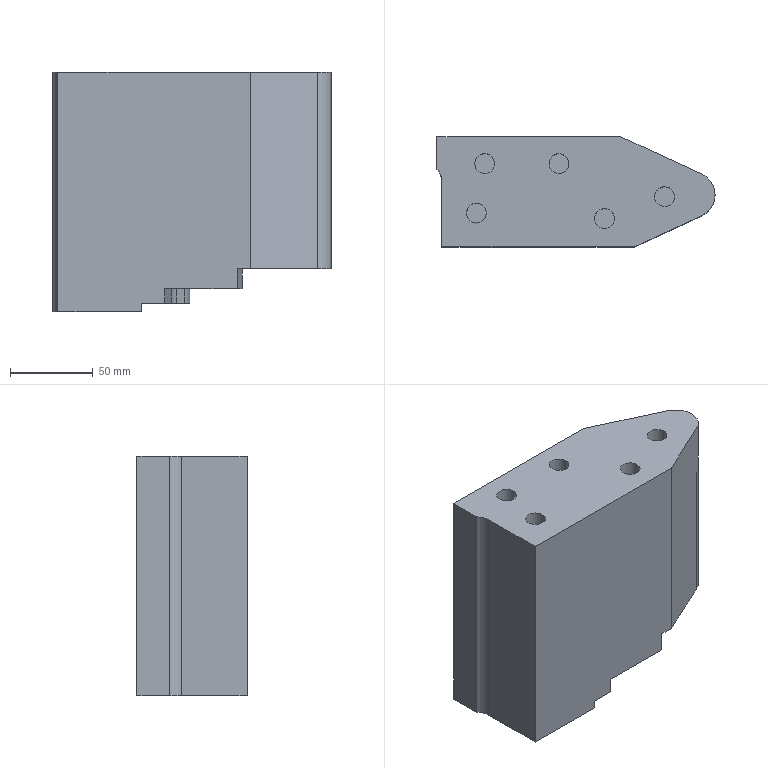Part | NX | features solid 2 | 1 solid | 34 faces | box 168.472 x 66.746 x 145 mm | volume 1281630 mm3 | plane 23 | cylinder 11 | commonest cylinder face diameters 12 x5 40 x4 20 x1 28 x1
STEP:
#1=CARTESIAN_POINT('',(645.,-7.,235.));
#2=VERTEX_POINT('',#1);
#3=CARTESIAN_POINT('',(645.,-13.,235.));
#4=DIRECTION('',(0.,0.,-1.));
#5=DIRECTION('',(0.,1.,0.));
#6=AXIS2_PLACEMENT_3D('',#3,#4,#5);
#7=CIRCLE('',#6,6.);
#8=EDGE_CURVE('',#2,#2,#7,.T.);
#9=ORIENTED_EDGE('',*,*,#8,.T.);
#10=EDGE_LOOP('',(#9));
#11=FACE_BOUND('',#10,.T.);
#12=CARTESIAN_POINT('',(650.,23.,235.));
#13=VERTEX_POINT('',#12);
#14=CARTESIAN_POINT('',(650.,17.,235.));
#15=DIRECTION('',(0.,0.,-1.));
#16=DIRECTION('',(0.,1.,0.));
#17=AXIS2_PLACEMENT_3D('',#14,#15,#16);
#18=CIRCLE('',#17,6.);
#19=EDGE_CURVE('',#13,#13,#18,.F.);
#20=ORIENTED_EDGE('',*,*,#19,.F.);
#21=EDGE_LOOP('',(#20));
#22=FACE_BOUND('',#21,.T.);
#23=CARTESIAN_POINT('',(695.,23.,235.));
#24=VERTEX_POINT('',#23);
#25=CARTESIAN_POINT('',(695.,17.,235.));
#26=DIRECTION('',(0.,0.,-1.));
#27=DIRECTION('',(0.,1.,0.));
#28=AXIS2_PLACEMENT_3D('',#25,#26,#27);
#29=CIRCLE('',#28,6.);
#30=EDGE_CURVE('',#24,#24,#29,.F.);
#31=ORIENTED_EDGE('',*,*,#30,.F.);
#32=EDGE_LOOP('',(#31));
#33=FACE_BOUND('',#32,.T.);
#34=CARTESIAN_POINT('',(722.608,-10.278,235.));
#35=VERTEX_POINT('',#34);
#36=CARTESIAN_POINT('',(722.608,-16.278,235.));
#37=DIRECTION('',(0.,0.,-1.));
#38=DIRECTION('',(0.,1.,0.));
#39=AXIS2_PLACEMENT_3D('',#36,#37,#38);
#40=CIRCLE('',#39,6.);
#41=EDGE_CURVE('',#35,#35,#40,.F.);
#42=ORIENTED_EDGE('',*,*,#41,.F.);
#43=EDGE_LOOP('',(#42));
#44=FACE_BOUND('',#43,.T.);
#45=CARTESIAN_POINT('',(759.,3.,235.));
#46=VERTEX_POINT('',#45);
#47=CARTESIAN_POINT('',(759.,-3.,235.));
#48=DIRECTION('',(0.,0.,-1.));
#49=DIRECTION('',(0.,1.,0.));
#50=AXIS2_PLACEMENT_3D('',#47,#48,#49);
#51=CIRCLE('',#50,6.);
#52=EDGE_CURVE('',#46,#46,#51,.F.);
#53=ORIENTED_EDGE('',*,*,#52,.F.);
#54=EDGE_LOOP('',(#53));
#55=FACE_BOUND('',#54,.T.);
#56=CARTESIAN_POINT('',(621.088,13.552,235.));
#57=VERTEX_POINT('',#56);
#58=CARTESIAN_POINT('',(621.088,33.298,235.));
#59=VERTEX_POINT('',#58);
#60=CARTESIAN_POINT('',(621.088,12.298,235.));
#61=DIRECTION('',(0.,1.,0.));
#62=VECTOR('',#61,1000.);
#63=LINE('',#60,#62);
#64=EDGE_CURVE('',#57,#59,#63,.T.);
#65=ORIENTED_EDGE('',*,*,#64,.F.);
#66=CARTESIAN_POINT('',(624.088,6.41,235.));
#67=VERTEX_POINT('',#66);
#68=CARTESIAN_POINT('',(614.088,6.41,235.));
#69=DIRECTION('',(0.,0.,-1.));
#70=DIRECTION('',(0.,1.,0.));
#71=AXIS2_PLACEMENT_3D('',#68,#69,#70);
#72=CIRCLE('',#71,10.);
#73=EDGE_CURVE('',#57,#67,#72,.T.);
#74=ORIENTED_EDGE('',*,*,#73,.T.);
#75=CARTESIAN_POINT('',(624.088,-33.448,235.));
#76=VERTEX_POINT('',#75);
#77=CARTESIAN_POINT('',(624.088,-164.676,235.));
#78=DIRECTION('',(0.,1.,0.));
#79=VECTOR('',#78,1000.);
#80=LINE('',#77,#79);
#81=EDGE_CURVE('',#67,#76,#80,.F.);
#82=ORIENTED_EDGE('',*,*,#81,.T.);
#83=CARTESIAN_POINT('',(740.626,-33.448,235.));
#84=VERTEX_POINT('',#83);
#85=CARTESIAN_POINT('',(-1135.,-33.448,235.));
#86=DIRECTION('',(-1.,0.,0.));
#87=VECTOR('',#86,1000.);
#88=LINE('',#85,#87);
#89=EDGE_CURVE('',#76,#84,#88,.F.);
#90=ORIENTED_EDGE('',*,*,#89,.T.);
#91=CARTESIAN_POINT('',(781.416,-14.665,235.));
#92=VERTEX_POINT('',#91);
#93=CARTESIAN_POINT('',(-856.712,-769.006,235.));
#94=DIRECTION('',(-0.9083,-0.4183,0.));
#95=VECTOR('',#94,1000.);
#96=LINE('',#93,#95);
#97=EDGE_CURVE('',#84,#92,#96,.F.);
#98=ORIENTED_EDGE('',*,*,#97,.T.);
#99=CARTESIAN_POINT('',(781.416,10.768,235.));
#100=VERTEX_POINT('',#99);
#101=CARTESIAN_POINT('',(775.56,-1.948,235.));
#102=DIRECTION('',(0.,0.,-1.));
#103=DIRECTION('',(0.,1.,0.));
#104=AXIS2_PLACEMENT_3D('',#101,#102,#103);
#105=CIRCLE('',#104,14.);
#106=EDGE_CURVE('',#92,#100,#105,.F.);
#107=ORIENTED_EDGE('',*,*,#106,.T.);
#108=CARTESIAN_POINT('',(732.491,33.298,235.));
#109=VERTEX_POINT('',#108);
#110=CARTESIAN_POINT('',(-733.063,708.17,235.));
#111=DIRECTION('',(0.9083,-0.4183,0.));
#112=VECTOR('',#111,1000.);
#113=LINE('',#110,#112);
#114=EDGE_CURVE('',#100,#109,#113,.F.);
#115=ORIENTED_EDGE('',*,*,#114,.T.);
#116=CARTESIAN_POINT('',(676.088,33.298,235.));
#117=DIRECTION('',(1.,0.,0.));
#118=VECTOR('',#117,1000.);
#119=LINE('',#116,#118);
#120=EDGE_CURVE('',#59,#109,#119,.T.);
#121=ORIENTED_EDGE('',*,*,#120,.F.);
#122=EDGE_LOOP('',(#65,#74,#82,#90,#98,#107,#115,#121));
#123=FACE_BOUND('',#122,.T.);
#124=CARTESIAN_POINT('',(-1135.,-164.676,235.));
#125=DIRECTION('',(0.,0.,-1.));
#126=DIRECTION('',(0.,1.,0.));
#127=AXIS2_PLACEMENT_3D('',#124,#125,#126);
#128=PLANE('',#127);
#129=ADVANCED_FACE('',(#11,#22,#33,#44,#55,#123),#128,.F.);
#130=ORIENTED_EDGE('',*,*,#89,.F.);
#131=CARTESIAN_POINT('',(624.088,-33.448,90.));
#132=VERTEX_POINT('',#131);
#133=CARTESIAN_POINT('',(624.088,-33.448,-185.));
#134=DIRECTION('',(0.,0.,1.));
#135=VECTOR('',#134,1000.);
#136=LINE('',#133,#135);
#137=EDGE_CURVE('',#132,#76,#136,.T.);
#138=ORIENTED_EDGE('',*,*,#137,.F.);
#139=CARTESIAN_POINT('',(674.638,-33.448,90.));
#140=VERTEX_POINT('',#139);
#141=CARTESIAN_POINT('',(621.088,-33.448,90.));
#142=DIRECTION('',(1.,0.,0.));
#143=VECTOR('',#142,1000.);
#144=LINE('',#141,#143);
#145=EDGE_CURVE('',#132,#140,#144,.T.);
#146=ORIENTED_EDGE('',*,*,#145,.T.);
#147=CARTESIAN_POINT('',(674.638,-33.448,95.));
#148=VERTEX_POINT('',#147);
#149=CARTESIAN_POINT('',(674.638,-33.448,95.));
#150=DIRECTION('',(0.,0.,-1.));
#151=VECTOR('',#150,1000.);
#152=LINE('',#149,#151);
#153=EDGE_CURVE('',#148,#140,#152,.T.);
#154=ORIENTED_EDGE('',*,*,#153,.F.);
#155=CARTESIAN_POINT('',(688.816,-33.448,95.));
#156=VERTEX_POINT('',#155);
#157=CARTESIAN_POINT('',(684.588,-33.448,95.));
#158=DIRECTION('',(1.,0.,0.));
#159=VECTOR('',#158,1000.);
#160=LINE('',#157,#159);
#161=EDGE_CURVE('',#148,#156,#160,.T.);
#162=ORIENTED_EDGE('',*,*,#161,.T.);
#163=CARTESIAN_POINT('',(688.816,-33.448,104.));
#164=VERTEX_POINT('',#163);
#165=CARTESIAN_POINT('',(688.816,-33.448,81.));
#166=DIRECTION('',(0.,0.,1.));
#167=VECTOR('',#166,1000.);
#168=LINE('',#165,#167);
#169=EDGE_CURVE('',#156,#164,#168,.T.);
#170=ORIENTED_EDGE('',*,*,#169,.T.);
#171=CARTESIAN_POINT('',(732.667,-33.448,104.));
#172=VERTEX_POINT('',#171);
#173=CARTESIAN_POINT('',(737.56,-33.448,104.));
#174=DIRECTION('',(-1.,0.,0.));
#175=VECTOR('',#174,1000.);
#176=LINE('',#173,#175);
#177=EDGE_CURVE('',#164,#172,#176,.F.);
#178=ORIENTED_EDGE('',*,*,#177,.T.);
#179=CARTESIAN_POINT('',(732.667,-33.448,116.));
#180=VERTEX_POINT('',#179);
#181=CARTESIAN_POINT('',(732.667,-33.448,81.));
#182=DIRECTION('',(0.,0.,1.));
#183=VECTOR('',#182,1000.);
#184=LINE('',#181,#183);
#185=EDGE_CURVE('',#172,#180,#184,.T.);
#186=ORIENTED_EDGE('',*,*,#185,.T.);
#187=CARTESIAN_POINT('',(740.626,-33.448,116.));
#188=VERTEX_POINT('',#187);
#189=CARTESIAN_POINT('',(737.56,-33.448,116.));
#190=DIRECTION('',(-1.,0.,0.));
#191=VECTOR('',#190,1000.);
#192=LINE('',#189,#191);
#193=EDGE_CURVE('',#180,#188,#192,.F.);
#194=ORIENTED_EDGE('',*,*,#193,.T.);
#195=CARTESIAN_POINT('',(740.626,-33.448,81.));
#196=DIRECTION('',(0.,0.,1.));
#197=VECTOR('',#196,1000.);
#198=LINE('',#195,#197);
#199=EDGE_CURVE('',#188,#84,#198,.T.);
#200=ORIENTED_EDGE('',*,*,#199,.T.);
#201=EDGE_LOOP('',(#130,#138,#146,#154,#162,#170,#178,#186,#194,#200));
#202=FACE_BOUND('',#201,.T.);
#203=CARTESIAN_POINT('',(737.56,-33.448,81.));
#204=DIRECTION('',(0.,-1.,0.));
#205=DIRECTION('',(0.,0.,1.));
#206=AXIS2_PLACEMENT_3D('',#203,#204,#205);
#207=PLANE('',#206);
#208=ADVANCED_FACE('',(#202),#207,.T.);
#209=CARTESIAN_POINT('',(621.088,13.552,90.));
#210=VERTEX_POINT('',#209);
#211=CARTESIAN_POINT('',(621.088,33.298,90.));
#212=VERTEX_POINT('',#211);
#213=CARTESIAN_POINT('',(621.088,-33.448,90.));
#214=DIRECTION('',(0.,1.,0.));
#215=VECTOR('',#214,1000.);
#216=LINE('',#213,#215);
#217=EDGE_CURVE('',#210,#212,#216,.T.);
#218=ORIENTED_EDGE('',*,*,#217,.F.);
#219=CARTESIAN_POINT('',(621.088,13.552,-185.));
#220=DIRECTION('',(0.,0.,1.));
#221=VECTOR('',#220,1000.);
#222=LINE('',#219,#221);
#223=EDGE_CURVE('',#210,#57,#222,.T.);
#224=ORIENTED_EDGE('',*,*,#223,.T.);
#225=ORIENTED_EDGE('',*,*,#64,.T.);
#226=CARTESIAN_POINT('',(621.088,33.298,95.));
#227=DIRECTION('',(0.,0.,1.));
#228=VECTOR('',#227,1000.);
#229=LINE('',#226,#228);
#230=EDGE_CURVE('',#212,#59,#229,.T.);
#231=ORIENTED_EDGE('',*,*,#230,.F.);
#232=EDGE_LOOP('',(#218,#224,#225,#231));
#233=FACE_BOUND('',#232,.T.);
#234=CARTESIAN_POINT('',(621.088,12.298,95.));
#235=DIRECTION('',(1.,0.,0.));
#236=DIRECTION('',(0.,1.,0.));
#237=AXIS2_PLACEMENT_3D('',#234,#235,#236);
#238=PLANE('',#237);
#239=ADVANCED_FACE('',(#233),#238,.F.);
#240=CARTESIAN_POINT('',(624.088,6.41,90.));
#241=VERTEX_POINT('',#240);
#242=CARTESIAN_POINT('',(614.088,6.41,90.));
#243=DIRECTION('',(0.,0.,1.));
#244=DIRECTION('',(1.,0.,0.));
#245=AXIS2_PLACEMENT_3D('',#242,#243,#244);
#246=CIRCLE('',#245,10.);
#247=EDGE_CURVE('',#210,#241,#246,.F.);
#248=ORIENTED_EDGE('',*,*,#247,.F.);
#249=ORIENTED_EDGE('',*,*,#217,.T.);
#250=CARTESIAN_POINT('',(650.299,33.298,90.));
#251=VERTEX_POINT('',#250);
#252=CARTESIAN_POINT('',(621.088,33.298,90.));
#253=DIRECTION('',(1.,0.,0.));
#254=VECTOR('',#253,1000.);
#255=LINE('',#252,#254);
#256=EDGE_CURVE('',#212,#251,#255,.T.);
#257=ORIENTED_EDGE('',*,*,#256,.T.);
#258=CARTESIAN_POINT('',(664.3,13.301,90.));
#259=VERTEX_POINT('',#258);
#260=CARTESIAN_POINT('',(649.897,33.871,90.));
#261=DIRECTION('',(0.5736,-0.8192,0.));
#262=VECTOR('',#261,1000.);
#263=LINE('',#260,#262);
#264=EDGE_CURVE('',#251,#259,#263,.T.);
#265=ORIENTED_EDGE('',*,*,#264,.T.);
#266=CARTESIAN_POINT('',(667.597,5.397,90.));
#267=VERTEX_POINT('',#266);
#268=CARTESIAN_POINT('',(647.917,1.829,90.));
#269=DIRECTION('',(0.,0.,1.));
#270=DIRECTION('',(1.,0.,0.));
#271=AXIS2_PLACEMENT_3D('',#268,#269,#270);
#272=CIRCLE('',#271,20.);
#273=EDGE_CURVE('',#259,#267,#272,.F.);
#274=ORIENTED_EDGE('',*,*,#273,.T.);
#275=CARTESIAN_POINT('',(666.854,9.494,90.));
#276=DIRECTION('',(0.1784,-0.984,0.));
#277=VECTOR('',#276,1000.);
#278=LINE('',#275,#277);
#279=EDGE_CURVE('',#267,#140,#278,.T.);
#280=ORIENTED_EDGE('',*,*,#279,.T.);
#281=ORIENTED_EDGE('',*,*,#145,.F.);
#282=CARTESIAN_POINT('',(624.088,-33.448,90.));
#283=DIRECTION('',(0.,-1.,0.));
#284=VECTOR('',#283,1000.);
#285=LINE('',#282,#284);
#286=EDGE_CURVE('',#241,#132,#285,.T.);
#287=ORIENTED_EDGE('',*,*,#286,.F.);
#288=EDGE_LOOP('',(#248,#249,#257,#265,#274,#280,#281,#287));
#289=FACE_BOUND('',#288,.T.);
#290=CARTESIAN_POINT('',(621.088,-33.448,90.));
#291=DIRECTION('',(0.,0.,1.));
#292=DIRECTION('',(1.,0.,0.));
#293=AXIS2_PLACEMENT_3D('',#290,#291,#292);
#294=PLANE('',#293);
#295=ADVANCED_FACE('',(#289),#294,.F.);
#296=CARTESIAN_POINT('',(704.088,33.298,95.));
#297=VERTEX_POINT('',#296);
#298=CARTESIAN_POINT('',(704.088,17.136,95.));
#299=VERTEX_POINT('',#298);
#300=CARTESIAN_POINT('',(704.088,-2.702,95.));
#301=DIRECTION('',(0.,-1.,0.));
#302=VECTOR('',#301,1000.);
#303=LINE('',#300,#302);
#304=EDGE_CURVE('',#297,#299,#303,.T.);
#305=ORIENTED_EDGE('',*,*,#304,.T.);
#306=CARTESIAN_POINT('',(700.722,6.031,95.));
#307=VERTEX_POINT('',#306);
#308=CARTESIAN_POINT('',(684.088,17.136,95.));
#309=DIRECTION('',(0.,0.,1.));
#310=DIRECTION('',(1.,0.,0.));
#311=AXIS2_PLACEMENT_3D('',#308,#309,#310);
#312=CIRCLE('',#311,20.);
#313=EDGE_CURVE('',#299,#307,#312,.F.);
#314=ORIENTED_EDGE('',*,*,#313,.T.);
#315=CARTESIAN_POINT('',(695.744,-1.427,95.));
#316=VERTEX_POINT('',#315);
#317=CARTESIAN_POINT('',(691.716,-7.46,95.));
#318=DIRECTION('',(0.5552,0.8317,0.));
#319=VECTOR('',#318,1000.);
#320=LINE('',#317,#319);
#321=EDGE_CURVE('',#316,#307,#320,.T.);
#322=ORIENTED_EDGE('',*,*,#321,.F.);
#323=CARTESIAN_POINT('',(692.624,-9.402,95.));
#324=VERTEX_POINT('',#323);
#325=CARTESIAN_POINT('',(712.378,-12.531,95.));
#326=DIRECTION('',(0.,0.,1.));
#327=DIRECTION('',(1.,0.,0.));
#328=AXIS2_PLACEMENT_3D('',#325,#326,#327);
#329=CIRCLE('',#328,20.);
#330=EDGE_CURVE('',#316,#324,#329,.T.);
#331=ORIENTED_EDGE('',*,*,#330,.T.);
#332=CARTESIAN_POINT('',(693.463,-4.108,95.));
#333=DIRECTION('',(0.1564,0.9877,0.));
#334=VECTOR('',#333,1000.);
#335=LINE('',#332,#334);
#336=EDGE_CURVE('',#156,#324,#335,.T.);
#337=ORIENTED_EDGE('',*,*,#336,.F.);
#338=ORIENTED_EDGE('',*,*,#161,.F.);
#339=CARTESIAN_POINT('',(667.597,5.397,95.));
#340=VERTEX_POINT('',#339);
#341=CARTESIAN_POINT('',(666.854,9.494,95.));
#342=DIRECTION('',(0.1784,-0.984,0.));
#343=VECTOR('',#342,1000.);
#344=LINE('',#341,#343);
#345=EDGE_CURVE('',#340,#148,#344,.T.);
#346=ORIENTED_EDGE('',*,*,#345,.F.);
#347=CARTESIAN_POINT('',(664.3,13.301,95.));
#348=VERTEX_POINT('',#347);
#349=CARTESIAN_POINT('',(647.917,1.829,95.));
#350=DIRECTION('',(0.,0.,1.));
#351=DIRECTION('',(1.,0.,0.));
#352=AXIS2_PLACEMENT_3D('',#349,#350,#351);
#353=CIRCLE('',#352,20.);
#354=EDGE_CURVE('',#340,#348,#353,.T.);
#355=ORIENTED_EDGE('',*,*,#354,.T.);
#356=CARTESIAN_POINT('',(650.299,33.298,95.));
#357=VERTEX_POINT('',#356);
#358=CARTESIAN_POINT('',(649.897,33.871,95.));
#359=DIRECTION('',(0.5736,-0.8192,0.));
#360=VECTOR('',#359,1000.);
#361=LINE('',#358,#360);
#362=EDGE_CURVE('',#357,#348,#361,.T.);
#363=ORIENTED_EDGE('',*,*,#362,.F.);
#364=CARTESIAN_POINT('',(676.088,33.298,95.));
#365=DIRECTION('',(-1.,0.,0.));
#366=VECTOR('',#365,1000.);
#367=LINE('',#364,#366);
#368=EDGE_CURVE('',#357,#297,#367,.F.);
#369=ORIENTED_EDGE('',*,*,#368,.T.);
#370=EDGE_LOOP('',(#305,#314,#322,#331,#337,#338,#346,#355,#363,#369));
#371=FACE_BOUND('',#370,.T.);
#372=CARTESIAN_POINT('',(684.588,-2.702,95.));
#373=DIRECTION('',(0.,0.,1.));
#374=DIRECTION('',(0.,1.,0.));
#375=AXIS2_PLACEMENT_3D('',#372,#373,#374);
#376=PLANE('',#375);
#377=ADVANCED_FACE('',(#371),#376,.F.);
#378=CARTESIAN_POINT('',(704.088,33.298,104.));
#379=VERTEX_POINT('',#378);
#380=CARTESIAN_POINT('',(704.088,33.298,95.));
#381=DIRECTION('',(0.,0.,-1.));
#382=VECTOR('',#381,1000.);
#383=LINE('',#380,#382);
#384=EDGE_CURVE('',#297,#379,#383,.F.);
#385=ORIENTED_EDGE('',*,*,#384,.F.);
#386=ORIENTED_EDGE('',*,*,#368,.F.);
#387=CARTESIAN_POINT('',(650.299,33.298,95.));
#388=DIRECTION('',(0.,0.,-1.));
#389=VECTOR('',#388,1000.);
#390=LINE('',#387,#389);
#391=EDGE_CURVE('',#357,#251,#390,.T.);
#392=ORIENTED_EDGE('',*,*,#391,.T.);
#393=ORIENTED_EDGE('',*,*,#256,.F.);
#394=ORIENTED_EDGE('',*,*,#230,.T.);
#395=ORIENTED_EDGE('',*,*,#120,.T.);
#396=CARTESIAN_POINT('',(732.491,33.298,116.));
#397=VERTEX_POINT('',#396);
#398=CARTESIAN_POINT('',(732.491,33.298,95.));
#399=DIRECTION('',(0.,0.,1.));
#400=VECTOR('',#399,1000.);
#401=LINE('',#398,#400);
#402=EDGE_CURVE('',#109,#397,#401,.F.);
#403=ORIENTED_EDGE('',*,*,#402,.T.);
#404=CARTESIAN_POINT('',(724.328,33.298,116.));
#405=VERTEX_POINT('',#404);
#406=CARTESIAN_POINT('',(676.088,33.298,116.));
#407=DIRECTION('',(-1.,0.,0.));
#408=VECTOR('',#407,1000.);
#409=LINE('',#406,#408);
#410=EDGE_CURVE('',#405,#397,#409,.F.);
#411=ORIENTED_EDGE('',*,*,#410,.F.);
#412=CARTESIAN_POINT('',(724.328,33.298,104.));
#413=VERTEX_POINT('',#412);
#414=CARTESIAN_POINT('',(724.328,33.298,95.));
#415=DIRECTION('',(0.,0.,1.));
#416=VECTOR('',#415,1000.);
#417=LINE('',#414,#416);
#418=EDGE_CURVE('',#413,#405,#417,.T.);
#419=ORIENTED_EDGE('',*,*,#418,.F.);
#420=CARTESIAN_POINT('',(718.314,33.298,104.));
#421=DIRECTION('',(1.,0.,0.));
#422=VECTOR('',#421,1000.);
#423=LINE('',#420,#422);
#424=EDGE_CURVE('',#379,#413,#423,.T.);
#425=ORIENTED_EDGE('',*,*,#424,.F.);
#426=EDGE_LOOP('',(#385,#386,#392,#393,#394,#395,#403,#411,#419,#425));
#427=FACE_BOUND('',#426,.T.);
#428=CARTESIAN_POINT('',(676.088,33.298,95.));
#429=DIRECTION('',(0.,-1.,0.));
#430=DIRECTION('',(1.,0.,0.));
#431=AXIS2_PLACEMENT_3D('',#428,#429,#430);
#432=PLANE('',#431);
#433=ADVANCED_FACE('',(#427),#432,.F.);
#434=CARTESIAN_POINT('',(781.416,-14.665,116.));
#435=VERTEX_POINT('',#434);
#436=CARTESIAN_POINT('',(781.416,-14.665,-270.));
#437=DIRECTION('',(0.,0.,1.));
#438=VECTOR('',#437,1000.);
#439=LINE('',#436,#438);
#440=EDGE_CURVE('',#435,#92,#439,.T.);
#441=ORIENTED_EDGE('',*,*,#440,.F.);
#442=CARTESIAN_POINT('',(781.416,10.768,116.));
#443=VERTEX_POINT('',#442);
#444=CARTESIAN_POINT('',(775.56,-1.948,116.));
#445=DIRECTION('',(0.,0.,1.));
#446=DIRECTION('',(1.,0.,0.));
#447=AXIS2_PLACEMENT_3D('',#444,#445,#446);
#448=CIRCLE('',#447,14.);
#449=EDGE_CURVE('',#435,#443,#448,.T.);
#450=ORIENTED_EDGE('',*,*,#449,.T.);
#451=CARTESIAN_POINT('',(781.416,10.768,-270.));
#452=DIRECTION('',(0.,0.,1.));
#453=VECTOR('',#452,1000.);
#454=LINE('',#451,#453);
#455=EDGE_CURVE('',#443,#100,#454,.T.);
#456=ORIENTED_EDGE('',*,*,#455,.T.);
#457=ORIENTED_EDGE('',*,*,#106,.F.);
#458=EDGE_LOOP('',(#441,#450,#456,#457));
#459=FACE_BOUND('',#458,.T.);
#460=CARTESIAN_POINT('',(775.56,-1.948,-270.));
#461=DIRECTION('',(0.,0.,1.));
#462=DIRECTION('',(1.,0.,0.));
#463=AXIS2_PLACEMENT_3D('',#460,#461,#462);
#464=CYLINDRICAL_SURFACE('',#463,14.);
#465=ADVANCED_FACE('',(#459),#464,.T.);
#466=CARTESIAN_POINT('',(758.397,21.368,116.));
#467=DIRECTION('',(-0.9083,0.4183,0.));
#468=VECTOR('',#467,1000.);
#469=LINE('',#466,#468);
#470=EDGE_CURVE('',#397,#443,#469,.F.);
#471=ORIENTED_EDGE('',*,*,#470,.F.);
#472=ORIENTED_EDGE('',*,*,#402,.F.);
#473=ORIENTED_EDGE('',*,*,#114,.F.);
#474=ORIENTED_EDGE('',*,*,#455,.F.);
#475=EDGE_LOOP('',(#471,#472,#473,#474));
#476=FACE_BOUND('',#475,.T.);
#477=CARTESIAN_POINT('',(781.416,10.768,-270.));
#478=DIRECTION('',(0.4183,0.9083,0.));
#479=DIRECTION('',(-0.9083,0.4183,0.));
#480=AXIS2_PLACEMENT_3D('',#477,#478,#479);
#481=PLANE('',#480);
#482=ADVANCED_FACE('',(#476),#481,.T.);
#483=ORIENTED_EDGE('',*,*,#199,.F.);
#484=CARTESIAN_POINT('',(781.416,-14.665,116.));
#485=DIRECTION('',(0.9083,0.4183,0.));
#486=VECTOR('',#485,1000.);
#487=LINE('',#484,#486);
#488=EDGE_CURVE('',#435,#188,#487,.F.);
#489=ORIENTED_EDGE('',*,*,#488,.F.);
#490=ORIENTED_EDGE('',*,*,#440,.T.);
#491=ORIENTED_EDGE('',*,*,#97,.F.);
#492=EDGE_LOOP('',(#483,#489,#490,#491));
#493=FACE_BOUND('',#492,.T.);
#494=CARTESIAN_POINT('',(736.614,-35.296,-270.));
#495=DIRECTION('',(0.4183,-0.9083,0.));
#496=DIRECTION('',(0.9083,0.4183,0.));
#497=AXIS2_PLACEMENT_3D('',#494,#495,#496);
#498=PLANE('',#497);
#499=ADVANCED_FACE('',(#493),#498,.T.);
#500=CARTESIAN_POINT('',(735.601,-16.808,104.));
#501=VERTEX_POINT('',#500);
#502=CARTESIAN_POINT('',(735.248,-8.251,104.));
#503=VERTEX_POINT('',#502);
#504=CARTESIAN_POINT('',(715.905,-13.335,104.));
#505=DIRECTION('',(0.,0.,1.));
#506=DIRECTION('',(1.,0.,0.));
#507=AXIS2_PLACEMENT_3D('',#504,#505,#506);
#508=CIRCLE('',#507,20.);
#509=EDGE_CURVE('',#501,#503,#508,.T.);
#510=ORIENTED_EDGE('',*,*,#509,.T.);
#511=CARTESIAN_POINT('',(735.248,-8.251,116.));
#512=VERTEX_POINT('',#511);
#513=CARTESIAN_POINT('',(735.248,-8.251,-384.));
#514=DIRECTION('',(0.,0.,1.));
#515=VECTOR('',#514,1000.);
#516=LINE('',#513,#515);
#517=EDGE_CURVE('',#503,#512,#516,.T.);
#518=ORIENTED_EDGE('',*,*,#517,.T.);
#519=CARTESIAN_POINT('',(735.601,-16.808,116.));
#520=VERTEX_POINT('',#519);
#521=CARTESIAN_POINT('',(715.905,-13.335,116.));
#522=DIRECTION('',(0.,0.,1.));
#523=DIRECTION('',(1.,0.,0.));
#524=AXIS2_PLACEMENT_3D('',#521,#522,#523);
#525=CIRCLE('',#524,20.);
#526=EDGE_CURVE('',#520,#512,#525,.T.);
#527=ORIENTED_EDGE('',*,*,#526,.F.);
#528=CARTESIAN_POINT('',(735.601,-16.808,-384.));
#529=DIRECTION('',(0.,0.,1.));
#530=VECTOR('',#529,1000.);
#531=LINE('',#528,#530);
#532=EDGE_CURVE('',#501,#520,#531,.T.);
#533=ORIENTED_EDGE('',*,*,#532,.F.);
#534=EDGE_LOOP('',(#510,#518,#527,#533));
#535=FACE_BOUND('',#534,.T.);
#536=CARTESIAN_POINT('',(715.905,-13.335,-384.));
#537=DIRECTION('',(0.,0.,1.));
#538=DIRECTION('',(1.,0.,0.));
#539=AXIS2_PLACEMENT_3D('',#536,#537,#538);
#540=CYLINDRICAL_SURFACE('',#539,20.);
#541=ADVANCED_FACE('',(#535),#540,.T.);
#542=CARTESIAN_POINT('',(736.303,-12.266,104.));
#543=DIRECTION('',(0.2542,-0.9672,0.));
#544=VECTOR('',#543,1000.);
#545=LINE('',#542,#544);
#546=EDGE_CURVE('',#503,#413,#545,.F.);
#547=ORIENTED_EDGE('',*,*,#546,.T.);
#548=ORIENTED_EDGE('',*,*,#418,.T.);
#549=CARTESIAN_POINT('',(736.303,-12.266,116.));
#550=DIRECTION('',(0.2542,-0.9672,0.));
#551=VECTOR('',#550,1000.);
#552=LINE('',#549,#551);
#553=EDGE_CURVE('',#512,#405,#552,.F.);
#554=ORIENTED_EDGE('',*,*,#553,.F.);
#555=ORIENTED_EDGE('',*,*,#517,.F.);
#556=EDGE_LOOP('',(#547,#548,#554,#555));
#557=FACE_BOUND('',#556,.T.);
#558=CARTESIAN_POINT('',(736.303,-12.266,-384.));
#559=DIRECTION('',(0.9672,0.2542,0.));
#560=DIRECTION('',(-0.2542,0.9672,0.));
#561=AXIS2_PLACEMENT_3D('',#558,#559,#560);
#562=PLANE('',#561);
#563=ADVANCED_FACE('',(#557),#562,.T.);
#564=CARTESIAN_POINT('',(739.347,4.437,104.));
#565=DIRECTION('',(-0.1736,-0.9848,0.));
#566=VECTOR('',#565,1000.);
#567=LINE('',#564,#566);
#568=EDGE_CURVE('',#172,#501,#567,.F.);
#569=ORIENTED_EDGE('',*,*,#568,.T.);
#570=ORIENTED_EDGE('',*,*,#532,.T.);
#571=CARTESIAN_POINT('',(739.347,4.437,116.));
#572=DIRECTION('',(-0.1736,-0.9848,0.));
#573=VECTOR('',#572,1000.);
#574=LINE('',#571,#573);
#575=EDGE_CURVE('',#180,#520,#574,.F.);
#576=ORIENTED_EDGE('',*,*,#575,.F.);
#577=ORIENTED_EDGE('',*,*,#185,.F.);
#578=EDGE_LOOP('',(#569,#570,#576,#577));
#579=FACE_BOUND('',#578,.T.);
#580=CARTESIAN_POINT('',(739.347,4.437,-384.));
#581=DIRECTION('',(0.9848,-0.1736,0.));
#582=DIRECTION('',(0.1736,0.9848,0.));
#583=AXIS2_PLACEMENT_3D('',#580,#581,#582);
#584=PLANE('',#583);
#585=ADVANCED_FACE('',(#579),#584,.T.);
#586=ORIENTED_EDGE('',*,*,#575,.T.);
#587=ORIENTED_EDGE('',*,*,#526,.T.);
#588=ORIENTED_EDGE('',*,*,#553,.T.);
#589=ORIENTED_EDGE('',*,*,#410,.T.);
#590=ORIENTED_EDGE('',*,*,#470,.T.);
#591=ORIENTED_EDGE('',*,*,#449,.F.);
#592=ORIENTED_EDGE('',*,*,#488,.T.);
#593=ORIENTED_EDGE('',*,*,#193,.F.);
#594=EDGE_LOOP('',(#586,#587,#588,#589,#590,#591,#592,#593));
#595=FACE_BOUND('',#594,.T.);
#596=CARTESIAN_POINT('',(775.56,-1.948,116.));
#597=DIRECTION('',(0.,0.,1.));
#598=DIRECTION('',(-1.,0.,0.));
#599=AXIS2_PLACEMENT_3D('',#596,#597,#598);
#600=PLANE('',#599);
#601=ADVANCED_FACE('',(#595),#600,.F.);
#602=ORIENTED_EDGE('',*,*,#279,.F.);
#603=CARTESIAN_POINT('',(667.597,5.397,95.));
#604=DIRECTION('',(0.,0.,-1.));
#605=VECTOR('',#604,1000.);
#606=LINE('',#603,#605);
#607=EDGE_CURVE('',#267,#340,#606,.F.);
#608=ORIENTED_EDGE('',*,*,#607,.T.);
#609=ORIENTED_EDGE('',*,*,#345,.T.);
#610=ORIENTED_EDGE('',*,*,#153,.T.);
#611=EDGE_LOOP('',(#602,#608,#609,#610));
#612=FACE_BOUND('',#611,.T.);
#613=CARTESIAN_POINT('',(666.854,9.494,95.));
#614=DIRECTION('',(0.984,0.1784,0.));
#615=DIRECTION('',(-0.1784,0.984,0.));
#616=AXIS2_PLACEMENT_3D('',#613,#614,#615);
#617=PLANE('',#616);
#618=ADVANCED_FACE('',(#612),#617,.T.);
#619=ORIENTED_EDGE('',*,*,#362,.T.);
#620=CARTESIAN_POINT('',(664.3,13.301,95.));
#621=DIRECTION('',(0.,0.,-1.));
#622=VECTOR('',#621,1000.);
#623=LINE('',#620,#622);
#624=EDGE_CURVE('',#348,#259,#623,.T.);
#625=ORIENTED_EDGE('',*,*,#624,.T.);
#626=ORIENTED_EDGE('',*,*,#264,.F.);
#627=ORIENTED_EDGE('',*,*,#391,.F.);
#628=EDGE_LOOP('',(#619,#625,#626,#627));
#629=FACE_BOUND('',#628,.T.);
#630=CARTESIAN_POINT('',(649.897,33.871,95.));
#631=DIRECTION('',(0.8192,0.5736,0.));
#632=DIRECTION('',(-0.5736,0.8192,0.));
#633=AXIS2_PLACEMENT_3D('',#630,#631,#632);
#634=PLANE('',#633);
#635=ADVANCED_FACE('',(#629),#634,.T.);
#636=ORIENTED_EDGE('',*,*,#354,.F.);
#637=ORIENTED_EDGE('',*,*,#607,.F.);
#638=ORIENTED_EDGE('',*,*,#273,.F.);
#639=ORIENTED_EDGE('',*,*,#624,.F.);
#640=EDGE_LOOP('',(#636,#637,#638,#639));
#641=FACE_BOUND('',#640,.T.);
#642=CARTESIAN_POINT('',(647.917,1.829,95.));
#643=DIRECTION('',(0.,0.,-1.));
#644=DIRECTION('',(-1.,0.,0.));
#645=AXIS2_PLACEMENT_3D('',#642,#643,#644);
#646=CYLINDRICAL_SURFACE('',#645,20.);
#647=ADVANCED_FACE('',(#641),#646,.T.);
#648=ORIENTED_EDGE('',*,*,#336,.T.);
#649=CARTESIAN_POINT('',(692.624,-9.402,104.));
#650=VERTEX_POINT('',#649);
#651=CARTESIAN_POINT('',(692.624,-9.402,104.));
#652=DIRECTION('',(0.,0.,1.));
#653=VECTOR('',#652,1000.);
#654=LINE('',#651,#653);
#655=EDGE_CURVE('',#324,#650,#654,.T.);
#656=ORIENTED_EDGE('',*,*,#655,.T.);
#657=CARTESIAN_POINT('',(688.84,-33.292,104.));
#658=DIRECTION('',(-0.1564,-0.9877,0.));
#659=VECTOR('',#658,1000.);
#660=LINE('',#657,#659);
#661=EDGE_CURVE('',#164,#650,#660,.F.);
#662=ORIENTED_EDGE('',*,*,#661,.F.);
#663=ORIENTED_EDGE('',*,*,#169,.F.);
#664=EDGE_LOOP('',(#648,#656,#662,#663));
#665=FACE_BOUND('',#664,.T.);
#666=CARTESIAN_POINT('',(688.84,-33.292,95.));
#667=DIRECTION('',(0.9877,-0.1564,0.));
#668=DIRECTION('',(0.1564,0.9877,0.));
#669=AXIS2_PLACEMENT_3D('',#666,#667,#668);
#670=PLANE('',#669);
#671=ADVANCED_FACE('',(#665),#670,.T.);
#672=ORIENTED_EDGE('',*,*,#321,.T.);
#673=CARTESIAN_POINT('',(700.722,6.031,104.));
#674=VERTEX_POINT('',#673);
#675=CARTESIAN_POINT('',(700.722,6.031,104.));
#676=DIRECTION('',(0.,0.,1.));
#677=VECTOR('',#676,1000.);
#678=LINE('',#675,#677);
#679=EDGE_CURVE('',#307,#674,#678,.T.);
#680=ORIENTED_EDGE('',*,*,#679,.T.);
#681=CARTESIAN_POINT('',(695.744,-1.427,104.));
#682=VERTEX_POINT('',#681);
#683=CARTESIAN_POINT('',(693.432,-4.89,104.));
#684=DIRECTION('',(-0.5552,-0.8317,0.));
#685=VECTOR('',#684,1000.);
#686=LINE('',#683,#685);
#687=EDGE_CURVE('',#682,#674,#686,.F.);
#688=ORIENTED_EDGE('',*,*,#687,.F.);
#689=CARTESIAN_POINT('',(695.744,-1.427,95.));
#690=DIRECTION('',(0.,0.,1.));
#691=VECTOR('',#690,1000.);
#692=LINE('',#689,#691);
#693=EDGE_CURVE('',#682,#316,#692,.F.);
#694=ORIENTED_EDGE('',*,*,#693,.T.);
#695=EDGE_LOOP('',(#672,#680,#688,#694));
#696=FACE_BOUND('',#695,.T.);
#697=CARTESIAN_POINT('',(693.432,-4.89,95.));
#698=DIRECTION('',(0.8317,-0.5552,0.));
#699=DIRECTION('',(0.5552,0.8317,0.));
#700=AXIS2_PLACEMENT_3D('',#697,#698,#699);
#701=PLANE('',#700);
#702=ADVANCED_FACE('',(#696),#701,.T.);
#703=ORIENTED_EDGE('',*,*,#661,.T.);
#704=CARTESIAN_POINT('',(712.378,-12.531,104.));
#705=DIRECTION('',(0.,0.,1.));
#706=DIRECTION('',(1.,0.,0.));
#707=AXIS2_PLACEMENT_3D('',#704,#705,#706);
#708=CIRCLE('',#707,20.);
#709=EDGE_CURVE('',#650,#682,#708,.F.);
#710=ORIENTED_EDGE('',*,*,#709,.T.);
#711=ORIENTED_EDGE('',*,*,#687,.T.);
#712=CARTESIAN_POINT('',(704.088,17.136,104.));
#713=VERTEX_POINT('',#712);
#714=CARTESIAN_POINT('',(684.088,17.136,104.));
#715=DIRECTION('',(0.,0.,1.));
#716=DIRECTION('',(1.,0.,0.));
#717=AXIS2_PLACEMENT_3D('',#714,#715,#716);
#718=CIRCLE('',#717,20.);
#719=EDGE_CURVE('',#674,#713,#718,.T.);
#720=ORIENTED_EDGE('',*,*,#719,.T.);
#721=CARTESIAN_POINT('',(704.088,33.298,104.));
#722=DIRECTION('',(0.,1.,0.));
#723=VECTOR('',#722,1000.);
#724=LINE('',#721,#723);
#725=EDGE_CURVE('',#379,#713,#724,.F.);
#726=ORIENTED_EDGE('',*,*,#725,.F.);
#727=ORIENTED_EDGE('',*,*,#424,.T.);
#728=ORIENTED_EDGE('',*,*,#546,.F.);
#729=ORIENTED_EDGE('',*,*,#509,.F.);
#730=ORIENTED_EDGE('',*,*,#568,.F.);
#731=ORIENTED_EDGE('',*,*,#177,.F.);
#732=EDGE_LOOP('',(#703,#710,#711,#720,#726,#727,#728,#729,#730,#731));
#733=FACE_BOUND('',#732,.T.);
#734=CARTESIAN_POINT('',(718.314,8.97,104.));
#735=DIRECTION('',(0.,0.,1.));
#736=DIRECTION('',(-0.1564,-0.9877,0.));
#737=AXIS2_PLACEMENT_3D('',#734,#735,#736);
#738=PLANE('',#737);
#739=ADVANCED_FACE('',(#733),#738,.F.);
#740=ORIENTED_EDGE('',*,*,#330,.F.);
#741=ORIENTED_EDGE('',*,*,#693,.F.);
#742=ORIENTED_EDGE('',*,*,#709,.F.);
#743=ORIENTED_EDGE('',*,*,#655,.F.);
#744=EDGE_LOOP('',(#740,#741,#742,#743));
#745=FACE_BOUND('',#744,.T.);
#746=CARTESIAN_POINT('',(712.378,-12.531,95.));
#747=DIRECTION('',(0.,0.,-1.));
#748=DIRECTION('',(-1.,0.,0.));
#749=AXIS2_PLACEMENT_3D('',#746,#747,#748);
#750=CYLINDRICAL_SURFACE('',#749,20.);
#751=ADVANCED_FACE('',(#745),#750,.F.);
#752=ORIENTED_EDGE('',*,*,#725,.T.);
#753=CARTESIAN_POINT('',(704.088,17.136,95.));
#754=DIRECTION('',(0.,0.,1.));
#755=VECTOR('',#754,1000.);
#756=LINE('',#753,#755);
#757=EDGE_CURVE('',#713,#299,#756,.F.);
#758=ORIENTED_EDGE('',*,*,#757,.T.);
#759=ORIENTED_EDGE('',*,*,#304,.F.);
#760=ORIENTED_EDGE('',*,*,#384,.T.);
#761=EDGE_LOOP('',(#752,#758,#759,#760));
#762=FACE_BOUND('',#761,.T.);
#763=CARTESIAN_POINT('',(704.088,33.298,95.));
#764=DIRECTION('',(-1.,0.,0.));
#765=DIRECTION('',(0.,0.,1.));
#766=AXIS2_PLACEMENT_3D('',#763,#764,#765);
#767=PLANE('',#766);
#768=ADVANCED_FACE('',(#762),#767,.F.);
#769=ORIENTED_EDGE('',*,*,#313,.F.);
#770=ORIENTED_EDGE('',*,*,#757,.F.);
#771=ORIENTED_EDGE('',*,*,#719,.F.);
#772=ORIENTED_EDGE('',*,*,#679,.F.);
#773=EDGE_LOOP('',(#769,#770,#771,#772));
#774=FACE_BOUND('',#773,.T.);
#775=CARTESIAN_POINT('',(684.088,17.136,95.));
#776=DIRECTION('',(0.,0.,-1.));
#777=DIRECTION('',(-1.,0.,0.));
#778=AXIS2_PLACEMENT_3D('',#775,#776,#777);
#779=CYLINDRICAL_SURFACE('',#778,20.);
#780=ADVANCED_FACE('',(#774),#779,.T.);
#781=ORIENTED_EDGE('',*,*,#19,.T.);
#782=EDGE_LOOP('',(#781));
#783=FACE_BOUND('',#782,.T.);
#784=CARTESIAN_POINT('',(650.,23.,185.));
#785=VERTEX_POINT('',#784);
#786=CARTESIAN_POINT('',(650.,17.,185.));
#787=DIRECTION('',(0.,0.,-1.));
#788=DIRECTION('',(0.,1.,0.));
#789=AXIS2_PLACEMENT_3D('',#786,#787,#788);
#790=CIRCLE('',#789,6.);
#791=EDGE_CURVE('',#785,#785,#790,.T.);
#792=ORIENTED_EDGE('',*,*,#791,.T.);
#793=EDGE_LOOP('',(#792));
#794=FACE_BOUND('',#793,.T.);
#795=CARTESIAN_POINT('',(650.,17.,285.));
#796=DIRECTION('',(0.,0.,-1.));
#797=DIRECTION('',(-1.,0.,0.));
#798=AXIS2_PLACEMENT_3D('',#795,#796,#797);
#799=CYLINDRICAL_SURFACE('',#798,6.);
#800=ADVANCED_FACE('',(#783,#794),#799,.F.);
#801=ORIENTED_EDGE('',*,*,#791,.F.);
#802=EDGE_LOOP('',(#801));
#803=FACE_BOUND('',#802,.T.);
#804=CARTESIAN_POINT('',(650.,17.,185.));
#805=DIRECTION('',(0.,0.,-1.));
#806=DIRECTION('',(-1.,0.,0.));
#807=AXIS2_PLACEMENT_3D('',#804,#805,#806);
#808=PLANE('',#807);
#809=ADVANCED_FACE('',(#803),#808,.F.);
#810=ORIENTED_EDGE('',*,*,#8,.F.);
#811=EDGE_LOOP('',(#810));
#812=FACE_BOUND('',#811,.T.);
#813=CARTESIAN_POINT('',(651.,-13.,185.));
#814=VERTEX_POINT('',#813);
#815=CARTESIAN_POINT('',(645.,-13.,185.));
#816=DIRECTION('',(0.,0.,1.));
#817=DIRECTION('',(1.,0.,0.));
#818=AXIS2_PLACEMENT_3D('',#815,#816,#817);
#819=CIRCLE('',#818,6.);
#820=EDGE_CURVE('',#814,#814,#819,.T.);
#821=ORIENTED_EDGE('',*,*,#820,.F.);
#822=EDGE_LOOP('',(#821));
#823=FACE_BOUND('',#822,.T.);
#824=CARTESIAN_POINT('',(645.,-13.,285.));
#825=DIRECTION('',(0.,0.,-1.));
#826=DIRECTION('',(-1.,0.,0.));
#827=AXIS2_PLACEMENT_3D('',#824,#825,#826);
#828=CYLINDRICAL_SURFACE('',#827,6.);
#829=ADVANCED_FACE('',(#812,#823),#828,.F.);
#830=ORIENTED_EDGE('',*,*,#820,.T.);
#831=EDGE_LOOP('',(#830));
#832=FACE_BOUND('',#831,.T.);
#833=CARTESIAN_POINT('',(645.,-13.,185.));
#834=DIRECTION('',(0.,0.,1.));
#835=DIRECTION('',(1.,0.,0.));
#836=AXIS2_PLACEMENT_3D('',#833,#834,#835);
#837=PLANE('',#836);
#838=ADVANCED_FACE('',(#832),#837,.T.);
#839=ORIENTED_EDGE('',*,*,#30,.T.);
#840=EDGE_LOOP('',(#839));
#841=FACE_BOUND('',#840,.T.);
#842=CARTESIAN_POINT('',(689.,17.,185.));
#843=VERTEX_POINT('',#842);
#844=CARTESIAN_POINT('',(695.,17.,185.));
#845=DIRECTION('',(0.,0.,-1.));
#846=DIRECTION('',(-1.,0.,0.));
#847=AXIS2_PLACEMENT_3D('',#844,#845,#846);
#848=CIRCLE('',#847,6.);
#849=EDGE_CURVE('',#843,#843,#848,.T.);
#850=ORIENTED_EDGE('',*,*,#849,.T.);
#851=EDGE_LOOP('',(#850));
#852=FACE_BOUND('',#851,.T.);
#853=CARTESIAN_POINT('',(695.,17.,285.));
#854=DIRECTION('',(0.,0.,-1.));
#855=DIRECTION('',(-1.,0.,0.));
#856=AXIS2_PLACEMENT_3D('',#853,#854,#855);
#857=CYLINDRICAL_SURFACE('',#856,6.);
#858=ADVANCED_FACE('',(#841,#852),#857,.F.);
#859=ORIENTED_EDGE('',*,*,#849,.F.);
#860=EDGE_LOOP('',(#859));
#861=FACE_BOUND('',#860,.T.);
#862=CARTESIAN_POINT('',(695.,17.,185.));
#863=DIRECTION('',(0.,0.,-1.));
#864=DIRECTION('',(-1.,0.,0.));
#865=AXIS2_PLACEMENT_3D('',#862,#863,#864);
#866=PLANE('',#865);
#867=ADVANCED_FACE('',(#861),#866,.F.);
#868=ORIENTED_EDGE('',*,*,#41,.T.);
#869=EDGE_LOOP('',(#868));
#870=FACE_BOUND('',#869,.T.);
#871=CARTESIAN_POINT('',(722.608,-10.278,185.));
#872=VERTEX_POINT('',#871);
#873=CARTESIAN_POINT('',(722.608,-16.278,185.));
#874=DIRECTION('',(0.,0.,-1.));
#875=DIRECTION('',(0.,1.,0.));
#876=AXIS2_PLACEMENT_3D('',#873,#874,#875);
#877=CIRCLE('',#876,6.);
#878=EDGE_CURVE('',#872,#872,#877,.T.);
#879=ORIENTED_EDGE('',*,*,#878,.T.);
#880=EDGE_LOOP('',(#879));
#881=FACE_BOUND('',#880,.T.);
#882=CARTESIAN_POINT('',(722.608,-16.278,285.));
#883=DIRECTION('',(0.,0.,-1.));
#884=DIRECTION('',(-1.,0.,0.));
#885=AXIS2_PLACEMENT_3D('',#882,#883,#884);
#886=CYLINDRICAL_SURFACE('',#885,6.);
#887=ADVANCED_FACE('',(#870,#881),#886,.F.);
#888=ORIENTED_EDGE('',*,*,#878,.F.);
#889=EDGE_LOOP('',(#888));
#890=FACE_BOUND('',#889,.T.);
#891=CARTESIAN_POINT('',(722.608,-16.278,185.));
#892=DIRECTION('',(0.,0.,-1.));
#893=DIRECTION('',(-1.,0.,0.));
#894=AXIS2_PLACEMENT_3D('',#891,#892,#893);
#895=PLANE('',#894);
#896=ADVANCED_FACE('',(#890),#895,.F.);
#897=ORIENTED_EDGE('',*,*,#52,.T.);
#898=EDGE_LOOP('',(#897));
#899=FACE_BOUND('',#898,.T.);
#900=CARTESIAN_POINT('',(753.,-3.,185.));
#901=VERTEX_POINT('',#900);
#902=CARTESIAN_POINT('',(759.,-3.,185.));
#903=DIRECTION('',(0.,0.,-1.));
#904=DIRECTION('',(-1.,0.,0.));
#905=AXIS2_PLACEMENT_3D('',#902,#903,#904);
#906=CIRCLE('',#905,6.);
#907=EDGE_CURVE('',#901,#901,#906,.T.);
#908=ORIENTED_EDGE('',*,*,#907,.T.);
#909=EDGE_LOOP('',(#908));
#910=FACE_BOUND('',#909,.T.);
#911=CARTESIAN_POINT('',(759.,-3.,285.));
#912=DIRECTION('',(0.,0.,-1.));
#913=DIRECTION('',(-1.,0.,0.));
#914=AXIS2_PLACEMENT_3D('',#911,#912,#913);
#915=CYLINDRICAL_SURFACE('',#914,6.);
#916=ADVANCED_FACE('',(#899,#910),#915,.F.);
#917=ORIENTED_EDGE('',*,*,#907,.F.);
#918=EDGE_LOOP('',(#917));
#919=FACE_BOUND('',#918,.T.);
#920=CARTESIAN_POINT('',(759.,-3.,185.));
#921=DIRECTION('',(0.,0.,-1.));
#922=DIRECTION('',(-1.,0.,0.));
#923=AXIS2_PLACEMENT_3D('',#920,#921,#922);
#924=PLANE('',#923);
#925=ADVANCED_FACE('',(#919),#924,.F.);
#926=ORIENTED_EDGE('',*,*,#223,.F.);
#927=ORIENTED_EDGE('',*,*,#247,.T.);
#928=CARTESIAN_POINT('',(624.088,6.41,-185.));
#929=DIRECTION('',(0.,0.,1.));
#930=VECTOR('',#929,1000.);
#931=LINE('',#928,#930);
#932=EDGE_CURVE('',#241,#67,#931,.T.);
#933=ORIENTED_EDGE('',*,*,#932,.T.);
#934=ORIENTED_EDGE('',*,*,#73,.F.);
#935=EDGE_LOOP('',(#926,#927,#933,#934));
#936=FACE_BOUND('',#935,.T.);
#937=CARTESIAN_POINT('',(614.088,6.41,-185.));
#938=DIRECTION('',(0.,0.,1.));
#939=DIRECTION('',(1.,0.,0.));
#940=AXIS2_PLACEMENT_3D('',#937,#938,#939);
#941=CYLINDRICAL_SURFACE('',#940,10.);
#942=ADVANCED_FACE('',(#936),#941,.F.);
#943=ORIENTED_EDGE('',*,*,#932,.F.);
#944=ORIENTED_EDGE('',*,*,#286,.T.);
#945=ORIENTED_EDGE('',*,*,#137,.T.);
#946=ORIENTED_EDGE('',*,*,#81,.F.);
#947=EDGE_LOOP('',(#943,#944,#945,#946));
#948=FACE_BOUND('',#947,.T.);
#949=CARTESIAN_POINT('',(624.088,6.41,-185.));
#950=DIRECTION('',(-1.,0.,0.));
#951=DIRECTION('',(0.,0.,1.));
#952=AXIS2_PLACEMENT_3D('',#949,#950,#951);
#953=PLANE('',#952);
#954=ADVANCED_FACE('',(#948),#953,.T.);
#955=CLOSED_SHELL('',(#129,#208,#239,#295,#377,#433,#465,#482,#499,#541,#563,#585,#601,#618,#635,#647,#671,#702,#739,#751,#768,#780,#800,#809,#829,#838,#858,#867,#887,#896,#916,#925,#942,#954));
#956=MANIFOLD_SOLID_BREP('',#955);
#957=(LENGTH_UNIT()NAMED_UNIT(*)SI_UNIT(.MILLI.,.METRE.));
#958=UNCERTAINTY_MEASURE_WITH_UNIT(LENGTH_MEASURE(0.00001),#957,'','');
#959=(NAMED_UNIT(*)PLANE_ANGLE_UNIT()SI_UNIT($,.RADIAN.));
#960=(NAMED_UNIT(*)SI_UNIT($,.STERADIAN.)SOLID_ANGLE_UNIT());
#961=(GEOMETRIC_REPRESENTATION_CONTEXT(3)GLOBAL_UNCERTAINTY_ASSIGNED_CONTEXT((#958))GLOBAL_UNIT_ASSIGNED_CONTEXT((#957,#959,#960))REPRESENTATION_CONTEXT('',''));
#962=ADVANCED_BREP_SHAPE_REPRESENTATION('',(#956),#961);